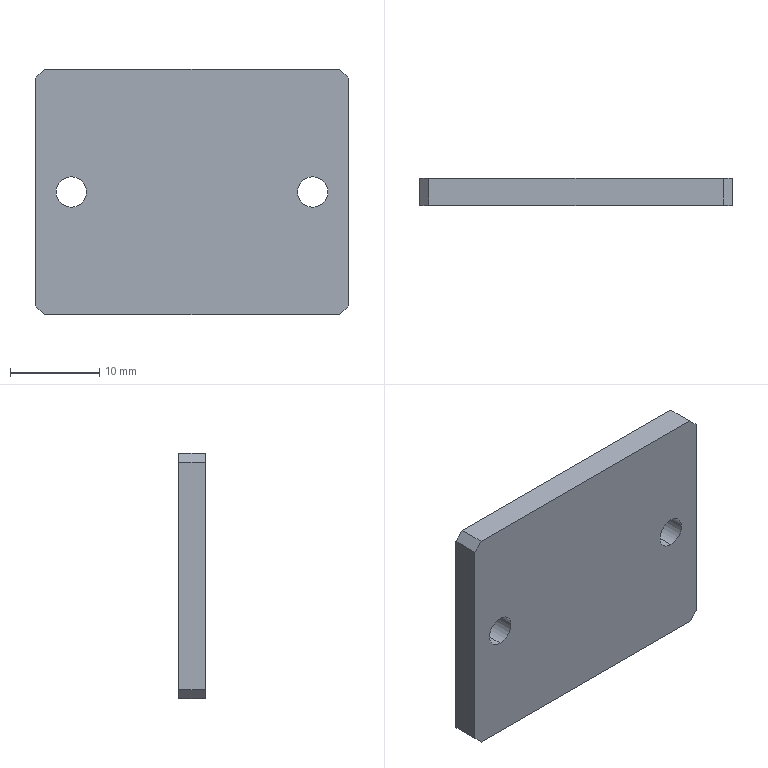Part | STEP file | PN_0050 | 1 solid | 14 faces | box 35 x 3 x 27.5 mm | volume 2827 mm3 | plane 10 | cylinder 4 | commonest cylinder face diameters 3.4 x4
STEP:
#1=CARTESIAN_POINT('',(0.,0.,0.));
#2=DIRECTION('',(0.,0.,1.));
#3=DIRECTION('',(1.,0.,0.));
#4=AXIS2_PLACEMENT_3D('',#1,#2,#3);
#5=CARTESIAN_POINT('',(13.5,0.,1.7));
#6=VERTEX_POINT('',#5);
#7=CARTESIAN_POINT('',(13.5,3.,1.7));
#8=VERTEX_POINT('',#7);
#9=CARTESIAN_POINT('',(13.5,0.,1.7));
#10=DIRECTION('',(0.,1.,0.));
#11=VECTOR('',#10,1.);
#12=LINE('',#9,#11);
#13=CARTESIAN_POINT('',(13.5,0.,0.));
#14=DIRECTION('',(0.,1.,0.));
#15=DIRECTION('',(0.,0.,1.));
#16=AXIS2_PLACEMENT_3D('',#13,#14,#15);
#17=CYLINDRICAL_SURFACE('',#16,1.7);
#18=CARTESIAN_POINT('',(6.283,0.));
#19=DIRECTION('',(0.,1.));
#20=VECTOR('',#19,1.);
#21=LINE('',#18,#20);
#22=(GEOMETRIC_REPRESENTATION_CONTEXT(2)PARAMETRIC_REPRESENTATION_CONTEXT()REPRESENTATION_CONTEXT('',''));
#23=DEFINITIONAL_REPRESENTATION('',(#21),#22);
#24=PCURVE('',#17,#23);
#25=CARTESIAN_POINT('',(13.5,0.,0.));
#26=DIRECTION('',(0.,1.,0.));
#27=DIRECTION('',(0.,0.,1.));
#28=AXIS2_PLACEMENT_3D('',#25,#26,#27);
#29=CYLINDRICAL_SURFACE('',#28,1.7);
#30=CARTESIAN_POINT('',(0.,0.));
#31=DIRECTION('',(0.,1.));
#32=VECTOR('',#31,1.);
#33=LINE('',#30,#32);
#34=(GEOMETRIC_REPRESENTATION_CONTEXT(2)PARAMETRIC_REPRESENTATION_CONTEXT()REPRESENTATION_CONTEXT('',''));
#35=DEFINITIONAL_REPRESENTATION('',(#33),#34);
#36=PCURVE('',#29,#35);
#37=SURFACE_CURVE('',#12,(#24,#36),.PCURVE_S1.);
#38=EDGE_CURVE('',#6,#8,#37,.T.);
#39=ORIENTED_EDGE('',*,*,#38,.T.);
#40=CARTESIAN_POINT('',(13.5,3.,-1.7));
#41=VERTEX_POINT('',#40);
#42=CARTESIAN_POINT('',(13.5,3.,0.));
#43=DIRECTION('',(0.,1.,0.));
#44=DIRECTION('',(0.,0.,1.));
#45=AXIS2_PLACEMENT_3D('',#42,#43,#44);
#46=CIRCLE('',#45,1.7);
#47=CARTESIAN_POINT('',(0.,3.));
#48=DIRECTION('',(1.,0.));
#49=VECTOR('',#48,1.);
#50=LINE('',#47,#49);
#51=(GEOMETRIC_REPRESENTATION_CONTEXT(2)PARAMETRIC_REPRESENTATION_CONTEXT()REPRESENTATION_CONTEXT('',''));
#52=DEFINITIONAL_REPRESENTATION('',(#50),#51);
#53=PCURVE('',#17,#52);
#54=CARTESIAN_POINT('',(0.,3.,0.));
#55=DIRECTION('',(0.,1.,0.));
#56=DIRECTION('',(0.,0.,1.));
#57=AXIS2_PLACEMENT_3D('',#54,#55,#56);
#58=PLANE('',#57);
#59=CARTESIAN_POINT('',(0.,13.5));
#60=DIRECTION('',(1.,0.));
#61=AXIS2_PLACEMENT_2D('',#59,#60);
#62=CIRCLE('',#61,1.7);
#63=(GEOMETRIC_REPRESENTATION_CONTEXT(2)PARAMETRIC_REPRESENTATION_CONTEXT()REPRESENTATION_CONTEXT('',''));
#64=DEFINITIONAL_REPRESENTATION('',(#62),#63);
#65=PCURVE('',#58,#64);
#66=SURFACE_CURVE('',#46,(#53,#65),.PCURVE_S1.);
#67=EDGE_CURVE('',#41,#8,#66,.T.);
#68=ORIENTED_EDGE('',*,*,#67,.F.);
#69=CARTESIAN_POINT('',(13.5,0.,-1.7));
#70=VERTEX_POINT('',#69);
#71=CARTESIAN_POINT('',(13.5,0.,-1.7));
#72=DIRECTION('',(0.,1.,0.));
#73=VECTOR('',#72,1.);
#74=LINE('',#71,#73);
#75=CARTESIAN_POINT('',(3.142,0.));
#76=DIRECTION('',(0.,1.));
#77=VECTOR('',#76,1.);
#78=LINE('',#75,#77);
#79=(GEOMETRIC_REPRESENTATION_CONTEXT(2)PARAMETRIC_REPRESENTATION_CONTEXT()REPRESENTATION_CONTEXT('',''));
#80=DEFINITIONAL_REPRESENTATION('',(#78),#79);
#81=PCURVE('',#17,#80);
#82=CARTESIAN_POINT('',(3.142,0.));
#83=DIRECTION('',(0.,1.));
#84=VECTOR('',#83,1.);
#85=LINE('',#82,#84);
#86=(GEOMETRIC_REPRESENTATION_CONTEXT(2)PARAMETRIC_REPRESENTATION_CONTEXT()REPRESENTATION_CONTEXT('',''));
#87=DEFINITIONAL_REPRESENTATION('',(#85),#86);
#88=PCURVE('',#29,#87);
#89=SURFACE_CURVE('',#74,(#81,#88),.PCURVE_S1.);
#90=EDGE_CURVE('',#70,#41,#89,.T.);
#91=ORIENTED_EDGE('',*,*,#90,.F.);
#92=CARTESIAN_POINT('',(13.5,0.,0.));
#93=DIRECTION('',(0.,1.,0.));
#94=DIRECTION('',(0.,0.,1.));
#95=AXIS2_PLACEMENT_3D('',#92,#93,#94);
#96=CIRCLE('',#95,1.7);
#97=CARTESIAN_POINT('',(0.,0.));
#98=DIRECTION('',(1.,0.));
#99=VECTOR('',#98,1.);
#100=LINE('',#97,#99);
#101=(GEOMETRIC_REPRESENTATION_CONTEXT(2)PARAMETRIC_REPRESENTATION_CONTEXT()REPRESENTATION_CONTEXT('',''));
#102=DEFINITIONAL_REPRESENTATION('',(#100),#101);
#103=PCURVE('',#17,#102);
#104=CARTESIAN_POINT('',(0.,0.,0.));
#105=DIRECTION('',(0.,1.,0.));
#106=DIRECTION('',(0.,0.,1.));
#107=AXIS2_PLACEMENT_3D('',#104,#105,#106);
#108=PLANE('',#107);
#109=CARTESIAN_POINT('',(0.,13.5));
#110=DIRECTION('',(1.,0.));
#111=AXIS2_PLACEMENT_2D('',#109,#110);
#112=CIRCLE('',#111,1.7);
#113=(GEOMETRIC_REPRESENTATION_CONTEXT(2)PARAMETRIC_REPRESENTATION_CONTEXT()REPRESENTATION_CONTEXT('',''));
#114=DEFINITIONAL_REPRESENTATION('',(#112),#113);
#115=PCURVE('',#108,#114);
#116=SURFACE_CURVE('',#96,(#103,#115),.PCURVE_S1.);
#117=EDGE_CURVE('',#70,#6,#116,.T.);
#118=ORIENTED_EDGE('',*,*,#117,.T.);
#119=EDGE_LOOP('',(#39,#68,#91,#118));
#120=FACE_BOUND('',#119,.F.);
#121=ADVANCED_FACE('',(#120),#17,.F.);
#122=CARTESIAN_POINT('',(-13.5,0.,1.7));
#123=VERTEX_POINT('',#122);
#124=CARTESIAN_POINT('',(-13.5,3.,1.7));
#125=VERTEX_POINT('',#124);
#126=CARTESIAN_POINT('',(-13.5,0.,1.7));
#127=DIRECTION('',(0.,1.,0.));
#128=VECTOR('',#127,1.);
#129=LINE('',#126,#128);
#130=CARTESIAN_POINT('',(-13.5,0.,0.));
#131=DIRECTION('',(0.,1.,0.));
#132=DIRECTION('',(0.,0.,1.));
#133=AXIS2_PLACEMENT_3D('',#130,#131,#132);
#134=CYLINDRICAL_SURFACE('',#133,1.7);
#135=CARTESIAN_POINT('',(6.283,0.));
#136=DIRECTION('',(0.,1.));
#137=VECTOR('',#136,1.);
#138=LINE('',#135,#137);
#139=(GEOMETRIC_REPRESENTATION_CONTEXT(2)PARAMETRIC_REPRESENTATION_CONTEXT()REPRESENTATION_CONTEXT('',''));
#140=DEFINITIONAL_REPRESENTATION('',(#138),#139);
#141=PCURVE('',#134,#140);
#142=CARTESIAN_POINT('',(-13.5,0.,0.));
#143=DIRECTION('',(0.,1.,0.));
#144=DIRECTION('',(0.,0.,1.));
#145=AXIS2_PLACEMENT_3D('',#142,#143,#144);
#146=CYLINDRICAL_SURFACE('',#145,1.7);
#147=CARTESIAN_POINT('',(0.,0.));
#148=DIRECTION('',(0.,1.));
#149=VECTOR('',#148,1.);
#150=LINE('',#147,#149);
#151=(GEOMETRIC_REPRESENTATION_CONTEXT(2)PARAMETRIC_REPRESENTATION_CONTEXT()REPRESENTATION_CONTEXT('',''));
#152=DEFINITIONAL_REPRESENTATION('',(#150),#151);
#153=PCURVE('',#146,#152);
#154=SURFACE_CURVE('',#129,(#141,#153),.PCURVE_S1.);
#155=EDGE_CURVE('',#123,#125,#154,.T.);
#156=ORIENTED_EDGE('',*,*,#155,.T.);
#157=CARTESIAN_POINT('',(-13.5,3.,-1.7));
#158=VERTEX_POINT('',#157);
#159=CARTESIAN_POINT('',(-13.5,3.,0.));
#160=DIRECTION('',(0.,1.,0.));
#161=DIRECTION('',(0.,0.,1.));
#162=AXIS2_PLACEMENT_3D('',#159,#160,#161);
#163=CIRCLE('',#162,1.7);
#164=CARTESIAN_POINT('',(0.,3.));
#165=DIRECTION('',(1.,0.));
#166=VECTOR('',#165,1.);
#167=LINE('',#164,#166);
#168=(GEOMETRIC_REPRESENTATION_CONTEXT(2)PARAMETRIC_REPRESENTATION_CONTEXT()REPRESENTATION_CONTEXT('',''));
#169=DEFINITIONAL_REPRESENTATION('',(#167),#168);
#170=PCURVE('',#134,#169);
#171=CARTESIAN_POINT('',(0.,-13.5));
#172=DIRECTION('',(1.,0.));
#173=AXIS2_PLACEMENT_2D('',#171,#172);
#174=CIRCLE('',#173,1.7);
#175=(GEOMETRIC_REPRESENTATION_CONTEXT(2)PARAMETRIC_REPRESENTATION_CONTEXT()REPRESENTATION_CONTEXT('',''));
#176=DEFINITIONAL_REPRESENTATION('',(#174),#175);
#177=PCURVE('',#58,#176);
#178=SURFACE_CURVE('',#163,(#170,#177),.PCURVE_S1.);
#179=EDGE_CURVE('',#158,#125,#178,.T.);
#180=ORIENTED_EDGE('',*,*,#179,.F.);
#181=CARTESIAN_POINT('',(-13.5,0.,-1.7));
#182=VERTEX_POINT('',#181);
#183=CARTESIAN_POINT('',(-13.5,0.,-1.7));
#184=DIRECTION('',(0.,1.,0.));
#185=VECTOR('',#184,1.);
#186=LINE('',#183,#185);
#187=CARTESIAN_POINT('',(3.142,0.));
#188=DIRECTION('',(0.,1.));
#189=VECTOR('',#188,1.);
#190=LINE('',#187,#189);
#191=(GEOMETRIC_REPRESENTATION_CONTEXT(2)PARAMETRIC_REPRESENTATION_CONTEXT()REPRESENTATION_CONTEXT('',''));
#192=DEFINITIONAL_REPRESENTATION('',(#190),#191);
#193=PCURVE('',#134,#192);
#194=CARTESIAN_POINT('',(3.142,0.));
#195=DIRECTION('',(0.,1.));
#196=VECTOR('',#195,1.);
#197=LINE('',#194,#196);
#198=(GEOMETRIC_REPRESENTATION_CONTEXT(2)PARAMETRIC_REPRESENTATION_CONTEXT()REPRESENTATION_CONTEXT('',''));
#199=DEFINITIONAL_REPRESENTATION('',(#197),#198);
#200=PCURVE('',#146,#199);
#201=SURFACE_CURVE('',#186,(#193,#200),.PCURVE_S1.);
#202=EDGE_CURVE('',#182,#158,#201,.T.);
#203=ORIENTED_EDGE('',*,*,#202,.F.);
#204=CARTESIAN_POINT('',(-13.5,0.,0.));
#205=DIRECTION('',(0.,1.,0.));
#206=DIRECTION('',(0.,0.,1.));
#207=AXIS2_PLACEMENT_3D('',#204,#205,#206);
#208=CIRCLE('',#207,1.7);
#209=CARTESIAN_POINT('',(0.,0.));
#210=DIRECTION('',(1.,0.));
#211=VECTOR('',#210,1.);
#212=LINE('',#209,#211);
#213=(GEOMETRIC_REPRESENTATION_CONTEXT(2)PARAMETRIC_REPRESENTATION_CONTEXT()REPRESENTATION_CONTEXT('',''));
#214=DEFINITIONAL_REPRESENTATION('',(#212),#213);
#215=PCURVE('',#134,#214);
#216=CARTESIAN_POINT('',(0.,-13.5));
#217=DIRECTION('',(1.,0.));
#218=AXIS2_PLACEMENT_2D('',#216,#217);
#219=CIRCLE('',#218,1.7);
#220=(GEOMETRIC_REPRESENTATION_CONTEXT(2)PARAMETRIC_REPRESENTATION_CONTEXT()REPRESENTATION_CONTEXT('',''));
#221=DEFINITIONAL_REPRESENTATION('',(#219),#220);
#222=PCURVE('',#108,#221);
#223=SURFACE_CURVE('',#208,(#215,#222),.PCURVE_S1.);
#224=EDGE_CURVE('',#182,#123,#223,.T.);
#225=ORIENTED_EDGE('',*,*,#224,.T.);
#226=EDGE_LOOP('',(#156,#180,#203,#225));
#227=FACE_BOUND('',#226,.F.);
#228=ADVANCED_FACE('',(#227),#134,.F.);
#229=CARTESIAN_POINT('',(17.5,0.,12.75));
#230=VERTEX_POINT('',#229);
#231=CARTESIAN_POINT('',(17.5,0.,-12.75));
#232=VERTEX_POINT('',#231);
#233=CARTESIAN_POINT('',(17.5,0.,-13.75));
#234=DIRECTION('',(0.,0.,-1.));
#235=VECTOR('',#234,1.);
#236=LINE('',#233,#235);
#237=CARTESIAN_POINT('',(17.5,3.,-13.75));
#238=DIRECTION('',(-1.,0.,0.));
#239=DIRECTION('',(0.,0.,1.));
#240=AXIS2_PLACEMENT_3D('',#237,#238,#239);
#241=PLANE('',#240);
#242=CARTESIAN_POINT('',(0.,-3.));
#243=DIRECTION('',(-1.,0.));
#244=VECTOR('',#243,1.);
#245=LINE('',#242,#244);
#246=(GEOMETRIC_REPRESENTATION_CONTEXT(2)PARAMETRIC_REPRESENTATION_CONTEXT()REPRESENTATION_CONTEXT('',''));
#247=DEFINITIONAL_REPRESENTATION('',(#245),#246);
#248=PCURVE('',#241,#247);
#249=CARTESIAN_POINT('',(-13.75,17.5));
#250=DIRECTION('',(-1.,0.));
#251=VECTOR('',#250,1.);
#252=LINE('',#249,#251);
#253=(GEOMETRIC_REPRESENTATION_CONTEXT(2)PARAMETRIC_REPRESENTATION_CONTEXT()REPRESENTATION_CONTEXT('',''));
#254=DEFINITIONAL_REPRESENTATION('',(#252),#253);
#255=PCURVE('',#108,#254);
#256=SURFACE_CURVE('',#236,(#248,#255),.PCURVE_S1.);
#257=EDGE_CURVE('',#230,#232,#256,.T.);
#258=ORIENTED_EDGE('',*,*,#257,.T.);
#259=CARTESIAN_POINT('',(17.5,3.,-12.75));
#260=VERTEX_POINT('',#259);
#261=CARTESIAN_POINT('',(17.5,3.,-12.75));
#262=DIRECTION('',(0.,1.,0.));
#263=VECTOR('',#262,1.);
#264=LINE('',#261,#263);
#265=CARTESIAN_POINT('',(1.,0.));
#266=DIRECTION('',(0.,1.));
#267=VECTOR('',#266,1.);
#268=LINE('',#265,#267);
#269=(GEOMETRIC_REPRESENTATION_CONTEXT(2)PARAMETRIC_REPRESENTATION_CONTEXT()REPRESENTATION_CONTEXT('',''));
#270=DEFINITIONAL_REPRESENTATION('',(#268),#269);
#271=PCURVE('',#241,#270);
#272=CARTESIAN_POINT('',(16.5,3.,-13.75));
#273=DIRECTION('',(-0.7071,0.,0.7071));
#274=DIRECTION('',(0.,-1.,0.));
#275=AXIS2_PLACEMENT_3D('',#272,#273,#274);
#276=PLANE('',#275);
#277=CARTESIAN_POINT('',(0.,1.414));
#278=DIRECTION('',(-1.,0.));
#279=VECTOR('',#278,1.);
#280=LINE('',#277,#279);
#281=(GEOMETRIC_REPRESENTATION_CONTEXT(2)PARAMETRIC_REPRESENTATION_CONTEXT()REPRESENTATION_CONTEXT('',''));
#282=DEFINITIONAL_REPRESENTATION('',(#280),#281);
#283=PCURVE('',#276,#282);
#284=SURFACE_CURVE('',#264,(#271,#283),.PCURVE_S1.);
#285=EDGE_CURVE('',#232,#260,#284,.T.);
#286=ORIENTED_EDGE('',*,*,#285,.T.);
#287=CARTESIAN_POINT('',(17.5,3.,12.75));
#288=VERTEX_POINT('',#287);
#289=CARTESIAN_POINT('',(17.5,3.,-13.75));
#290=DIRECTION('',(0.,0.,-1.));
#291=VECTOR('',#290,1.);
#292=LINE('',#289,#291);
#293=CARTESIAN_POINT('',(0.,0.));
#294=DIRECTION('',(-1.,0.));
#295=VECTOR('',#294,1.);
#296=LINE('',#293,#295);
#297=(GEOMETRIC_REPRESENTATION_CONTEXT(2)PARAMETRIC_REPRESENTATION_CONTEXT()REPRESENTATION_CONTEXT('',''));
#298=DEFINITIONAL_REPRESENTATION('',(#296),#297);
#299=PCURVE('',#241,#298);
#300=CARTESIAN_POINT('',(-13.75,17.5));
#301=DIRECTION('',(-1.,0.));
#302=VECTOR('',#301,1.);
#303=LINE('',#300,#302);
#304=(GEOMETRIC_REPRESENTATION_CONTEXT(2)PARAMETRIC_REPRESENTATION_CONTEXT()REPRESENTATION_CONTEXT('',''));
#305=DEFINITIONAL_REPRESENTATION('',(#303),#304);
#306=PCURVE('',#58,#305);
#307=SURFACE_CURVE('',#292,(#299,#306),.PCURVE_S1.);
#308=EDGE_CURVE('',#288,#260,#307,.T.);
#309=ORIENTED_EDGE('',*,*,#308,.F.);
#310=CARTESIAN_POINT('',(17.5,3.,12.75));
#311=DIRECTION('',(0.,-1.,0.));
#312=VECTOR('',#311,1.);
#313=LINE('',#310,#312);
#314=CARTESIAN_POINT('',(26.5,0.));
#315=DIRECTION('',(0.,-1.));
#316=VECTOR('',#315,1.);
#317=LINE('',#314,#316);
#318=(GEOMETRIC_REPRESENTATION_CONTEXT(2)PARAMETRIC_REPRESENTATION_CONTEXT()REPRESENTATION_CONTEXT('',''));
#319=DEFINITIONAL_REPRESENTATION('',(#317),#318);
#320=PCURVE('',#241,#319);
#321=CARTESIAN_POINT('',(17.5,3.,12.75));
#322=DIRECTION('',(-0.7071,0.,-0.7071));
#323=DIRECTION('',(0.,-1.,0.));
#324=AXIS2_PLACEMENT_3D('',#321,#322,#323);
#325=PLANE('',#324);
#326=CARTESIAN_POINT('',(0.,0.));
#327=DIRECTION('',(1.,0.));
#328=VECTOR('',#327,1.);
#329=LINE('',#326,#328);
#330=(GEOMETRIC_REPRESENTATION_CONTEXT(2)PARAMETRIC_REPRESENTATION_CONTEXT()REPRESENTATION_CONTEXT('',''));
#331=DEFINITIONAL_REPRESENTATION('',(#329),#330);
#332=PCURVE('',#325,#331);
#333=SURFACE_CURVE('',#313,(#320,#332),.PCURVE_S1.);
#334=EDGE_CURVE('',#288,#230,#333,.T.);
#335=ORIENTED_EDGE('',*,*,#334,.T.);
#336=EDGE_LOOP('',(#258,#286,#309,#335));
#337=FACE_BOUND('',#336,.T.);
#338=ADVANCED_FACE('',(#337),#241,.F.);
#339=CARTESIAN_POINT('',(16.5,3.,-13.75));
#340=VERTEX_POINT('',#339);
#341=CARTESIAN_POINT('',(-16.5,3.,-13.75));
#342=VERTEX_POINT('',#341);
#343=CARTESIAN_POINT('',(-17.5,3.,-13.75));
#344=DIRECTION('',(-1.,0.,0.));
#345=VECTOR('',#344,1.);
#346=LINE('',#343,#345);
#347=CARTESIAN_POINT('',(-17.5,3.,-13.75));
#348=DIRECTION('',(0.,0.,1.));
#349=DIRECTION('',(1.,0.,0.));
#350=AXIS2_PLACEMENT_3D('',#347,#348,#349);
#351=PLANE('',#350);
#352=CARTESIAN_POINT('',(0.,0.));
#353=DIRECTION('',(-1.,0.));
#354=VECTOR('',#353,1.);
#355=LINE('',#352,#354);
#356=(GEOMETRIC_REPRESENTATION_CONTEXT(2)PARAMETRIC_REPRESENTATION_CONTEXT()REPRESENTATION_CONTEXT('',''));
#357=DEFINITIONAL_REPRESENTATION('',(#355),#356);
#358=PCURVE('',#351,#357);
#359=CARTESIAN_POINT('',(-13.75,-17.5));
#360=DIRECTION('',(0.,-1.));
#361=VECTOR('',#360,1.);
#362=LINE('',#359,#361);
#363=(GEOMETRIC_REPRESENTATION_CONTEXT(2)PARAMETRIC_REPRESENTATION_CONTEXT()REPRESENTATION_CONTEXT('',''));
#364=DEFINITIONAL_REPRESENTATION('',(#362),#363);
#365=PCURVE('',#58,#364);
#366=SURFACE_CURVE('',#346,(#358,#365),.PCURVE_S1.);
#367=EDGE_CURVE('',#340,#342,#366,.T.);
#368=ORIENTED_EDGE('',*,*,#367,.F.);
#369=CARTESIAN_POINT('',(16.5,0.,-13.75));
#370=VERTEX_POINT('',#369);
#371=CARTESIAN_POINT('',(16.5,3.,-13.75));
#372=DIRECTION('',(0.,-1.,0.));
#373=VECTOR('',#372,1.);
#374=LINE('',#371,#373);
#375=CARTESIAN_POINT('',(34.,0.));
#376=DIRECTION('',(0.,-1.));
#377=VECTOR('',#376,1.);
#378=LINE('',#375,#377);
#379=(GEOMETRIC_REPRESENTATION_CONTEXT(2)PARAMETRIC_REPRESENTATION_CONTEXT()REPRESENTATION_CONTEXT('',''));
#380=DEFINITIONAL_REPRESENTATION('',(#378),#379);
#381=PCURVE('',#351,#380);
#382=CARTESIAN_POINT('',(0.,0.));
#383=DIRECTION('',(1.,0.));
#384=VECTOR('',#383,1.);
#385=LINE('',#382,#384);
#386=(GEOMETRIC_REPRESENTATION_CONTEXT(2)PARAMETRIC_REPRESENTATION_CONTEXT()REPRESENTATION_CONTEXT('',''));
#387=DEFINITIONAL_REPRESENTATION('',(#385),#386);
#388=PCURVE('',#276,#387);
#389=SURFACE_CURVE('',#374,(#381,#388),.PCURVE_S1.);
#390=EDGE_CURVE('',#340,#370,#389,.T.);
#391=ORIENTED_EDGE('',*,*,#390,.T.);
#392=CARTESIAN_POINT('',(-16.5,0.,-13.75));
#393=VERTEX_POINT('',#392);
#394=CARTESIAN_POINT('',(-17.5,0.,-13.75));
#395=DIRECTION('',(-1.,0.,0.));
#396=VECTOR('',#395,1.);
#397=LINE('',#394,#396);
#398=CARTESIAN_POINT('',(0.,-3.));
#399=DIRECTION('',(-1.,0.));
#400=VECTOR('',#399,1.);
#401=LINE('',#398,#400);
#402=(GEOMETRIC_REPRESENTATION_CONTEXT(2)PARAMETRIC_REPRESENTATION_CONTEXT()REPRESENTATION_CONTEXT('',''));
#403=DEFINITIONAL_REPRESENTATION('',(#401),#402);
#404=PCURVE('',#351,#403);
#405=CARTESIAN_POINT('',(-13.75,-17.5));
#406=DIRECTION('',(0.,-1.));
#407=VECTOR('',#406,1.);
#408=LINE('',#405,#407);
#409=(GEOMETRIC_REPRESENTATION_CONTEXT(2)PARAMETRIC_REPRESENTATION_CONTEXT()REPRESENTATION_CONTEXT('',''));
#410=DEFINITIONAL_REPRESENTATION('',(#408),#409);
#411=PCURVE('',#108,#410);
#412=SURFACE_CURVE('',#397,(#404,#411),.PCURVE_S1.);
#413=EDGE_CURVE('',#370,#393,#412,.T.);
#414=ORIENTED_EDGE('',*,*,#413,.T.);
#415=CARTESIAN_POINT('',(-16.5,3.,-13.75));
#416=DIRECTION('',(0.,1.,0.));
#417=VECTOR('',#416,1.);
#418=LINE('',#415,#417);
#419=CARTESIAN_POINT('',(1.,0.));
#420=DIRECTION('',(0.,1.));
#421=VECTOR('',#420,1.);
#422=LINE('',#419,#421);
#423=(GEOMETRIC_REPRESENTATION_CONTEXT(2)PARAMETRIC_REPRESENTATION_CONTEXT()REPRESENTATION_CONTEXT('',''));
#424=DEFINITIONAL_REPRESENTATION('',(#422),#423);
#425=PCURVE('',#351,#424);
#426=CARTESIAN_POINT('',(-17.5,3.,-12.75));
#427=DIRECTION('',(0.7071,0.,0.7071));
#428=DIRECTION('',(0.,-1.,0.));
#429=AXIS2_PLACEMENT_3D('',#426,#427,#428);
#430=PLANE('',#429);
#431=CARTESIAN_POINT('',(0.,1.414));
#432=DIRECTION('',(-1.,0.));
#433=VECTOR('',#432,1.);
#434=LINE('',#431,#433);
#435=(GEOMETRIC_REPRESENTATION_CONTEXT(2)PARAMETRIC_REPRESENTATION_CONTEXT()REPRESENTATION_CONTEXT('',''));
#436=DEFINITIONAL_REPRESENTATION('',(#434),#435);
#437=PCURVE('',#430,#436);
#438=SURFACE_CURVE('',#418,(#425,#437),.PCURVE_S1.);
#439=EDGE_CURVE('',#393,#342,#438,.T.);
#440=ORIENTED_EDGE('',*,*,#439,.T.);
#441=EDGE_LOOP('',(#368,#391,#414,#440));
#442=FACE_BOUND('',#441,.T.);
#443=ADVANCED_FACE('',(#442),#351,.F.);
#444=CARTESIAN_POINT('',(-17.5,3.,-12.75));
#445=VERTEX_POINT('',#444);
#446=CARTESIAN_POINT('',(-17.5,3.,12.75));
#447=VERTEX_POINT('',#446);
#448=CARTESIAN_POINT('',(-17.5,3.,-13.75));
#449=DIRECTION('',(0.,0.,1.));
#450=VECTOR('',#449,1.);
#451=LINE('',#448,#450);
#452=CARTESIAN_POINT('',(-17.5,3.,-13.75));
#453=DIRECTION('',(1.,0.,0.));
#454=DIRECTION('',(0.,0.,-1.));
#455=AXIS2_PLACEMENT_3D('',#452,#453,#454);
#456=PLANE('',#455);
#457=CARTESIAN_POINT('',(0.,0.));
#458=DIRECTION('',(-1.,0.));
#459=VECTOR('',#458,1.);
#460=LINE('',#457,#459);
#461=(GEOMETRIC_REPRESENTATION_CONTEXT(2)PARAMETRIC_REPRESENTATION_CONTEXT()REPRESENTATION_CONTEXT('',''));
#462=DEFINITIONAL_REPRESENTATION('',(#460),#461);
#463=PCURVE('',#456,#462);
#464=CARTESIAN_POINT('',(-13.75,-17.5));
#465=DIRECTION('',(1.,0.));
#466=VECTOR('',#465,1.);
#467=LINE('',#464,#466);
#468=(GEOMETRIC_REPRESENTATION_CONTEXT(2)PARAMETRIC_REPRESENTATION_CONTEXT()REPRESENTATION_CONTEXT('',''));
#469=DEFINITIONAL_REPRESENTATION('',(#467),#468);
#470=PCURVE('',#58,#469);
#471=SURFACE_CURVE('',#451,(#463,#470),.PCURVE_S1.);
#472=EDGE_CURVE('',#445,#447,#471,.T.);
#473=ORIENTED_EDGE('',*,*,#472,.F.);
#474=CARTESIAN_POINT('',(-17.5,0.,-12.75));
#475=VERTEX_POINT('',#474);
#476=CARTESIAN_POINT('',(-17.5,3.,-12.75));
#477=DIRECTION('',(0.,-1.,0.));
#478=VECTOR('',#477,1.);
#479=LINE('',#476,#478);
#480=CARTESIAN_POINT('',(-1.,0.));
#481=DIRECTION('',(0.,-1.));
#482=VECTOR('',#481,1.);
#483=LINE('',#480,#482);
#484=(GEOMETRIC_REPRESENTATION_CONTEXT(2)PARAMETRIC_REPRESENTATION_CONTEXT()REPRESENTATION_CONTEXT('',''));
#485=DEFINITIONAL_REPRESENTATION('',(#483),#484);
#486=PCURVE('',#456,#485);
#487=CARTESIAN_POINT('',(0.,0.));
#488=DIRECTION('',(1.,0.));
#489=VECTOR('',#488,1.);
#490=LINE('',#487,#489);
#491=(GEOMETRIC_REPRESENTATION_CONTEXT(2)PARAMETRIC_REPRESENTATION_CONTEXT()REPRESENTATION_CONTEXT('',''));
#492=DEFINITIONAL_REPRESENTATION('',(#490),#491);
#493=PCURVE('',#430,#492);
#494=SURFACE_CURVE('',#479,(#486,#493),.PCURVE_S1.);
#495=EDGE_CURVE('',#445,#475,#494,.T.);
#496=ORIENTED_EDGE('',*,*,#495,.T.);
#497=CARTESIAN_POINT('',(-17.5,0.,12.75));
#498=VERTEX_POINT('',#497);
#499=CARTESIAN_POINT('',(-17.5,0.,-13.75));
#500=DIRECTION('',(0.,0.,1.));
#501=VECTOR('',#500,1.);
#502=LINE('',#499,#501);
#503=CARTESIAN_POINT('',(0.,-3.));
#504=DIRECTION('',(-1.,0.));
#505=VECTOR('',#504,1.);
#506=LINE('',#503,#505);
#507=(GEOMETRIC_REPRESENTATION_CONTEXT(2)PARAMETRIC_REPRESENTATION_CONTEXT()REPRESENTATION_CONTEXT('',''));
#508=DEFINITIONAL_REPRESENTATION('',(#506),#507);
#509=PCURVE('',#456,#508);
#510=CARTESIAN_POINT('',(-13.75,-17.5));
#511=DIRECTION('',(1.,0.));
#512=VECTOR('',#511,1.);
#513=LINE('',#510,#512);
#514=(GEOMETRIC_REPRESENTATION_CONTEXT(2)PARAMETRIC_REPRESENTATION_CONTEXT()REPRESENTATION_CONTEXT('',''));
#515=DEFINITIONAL_REPRESENTATION('',(#513),#514);
#516=PCURVE('',#108,#515);
#517=SURFACE_CURVE('',#502,(#509,#516),.PCURVE_S1.);
#518=EDGE_CURVE('',#475,#498,#517,.T.);
#519=ORIENTED_EDGE('',*,*,#518,.T.);
#520=CARTESIAN_POINT('',(-17.5,3.,12.75));
#521=DIRECTION('',(0.,1.,0.));
#522=VECTOR('',#521,1.);
#523=LINE('',#520,#522);
#524=CARTESIAN_POINT('',(-26.5,0.));
#525=DIRECTION('',(0.,1.));
#526=VECTOR('',#525,1.);
#527=LINE('',#524,#526);
#528=(GEOMETRIC_REPRESENTATION_CONTEXT(2)PARAMETRIC_REPRESENTATION_CONTEXT()REPRESENTATION_CONTEXT('',''));
#529=DEFINITIONAL_REPRESENTATION('',(#527),#528);
#530=PCURVE('',#456,#529);
#531=CARTESIAN_POINT('',(-16.5,3.,13.75));
#532=DIRECTION('',(0.7071,0.,-0.7071));
#533=DIRECTION('',(0.,-1.,0.));
#534=AXIS2_PLACEMENT_3D('',#531,#532,#533);
#535=PLANE('',#534);
#536=CARTESIAN_POINT('',(0.,1.414));
#537=DIRECTION('',(-1.,0.));
#538=VECTOR('',#537,1.);
#539=LINE('',#536,#538);
#540=(GEOMETRIC_REPRESENTATION_CONTEXT(2)PARAMETRIC_REPRESENTATION_CONTEXT()REPRESENTATION_CONTEXT('',''));
#541=DEFINITIONAL_REPRESENTATION('',(#539),#540);
#542=PCURVE('',#535,#541);
#543=SURFACE_CURVE('',#523,(#530,#542),.PCURVE_S1.);
#544=EDGE_CURVE('',#498,#447,#543,.T.);
#545=ORIENTED_EDGE('',*,*,#544,.T.);
#546=EDGE_LOOP('',(#473,#496,#519,#545));
#547=FACE_BOUND('',#546,.T.);
#548=ADVANCED_FACE('',(#547),#456,.F.);
#549=CARTESIAN_POINT('',(-16.5,0.,13.75));
#550=VERTEX_POINT('',#549);
#551=CARTESIAN_POINT('',(16.5,0.,13.75));
#552=VERTEX_POINT('',#551);
#553=CARTESIAN_POINT('',(-17.5,0.,13.75));
#554=DIRECTION('',(1.,0.,0.));
#555=VECTOR('',#554,1.);
#556=LINE('',#553,#555);
#557=CARTESIAN_POINT('',(-17.5,3.,13.75));
#558=DIRECTION('',(0.,0.,-1.));
#559=DIRECTION('',(-1.,0.,0.));
#560=AXIS2_PLACEMENT_3D('',#557,#558,#559);
#561=PLANE('',#560);
#562=CARTESIAN_POINT('',(0.,-3.));
#563=DIRECTION('',(-1.,0.));
#564=VECTOR('',#563,1.);
#565=LINE('',#562,#564);
#566=(GEOMETRIC_REPRESENTATION_CONTEXT(2)PARAMETRIC_REPRESENTATION_CONTEXT()REPRESENTATION_CONTEXT('',''));
#567=DEFINITIONAL_REPRESENTATION('',(#565),#566);
#568=PCURVE('',#561,#567);
#569=CARTESIAN_POINT('',(13.75,-17.5));
#570=DIRECTION('',(0.,1.));
#571=VECTOR('',#570,1.);
#572=LINE('',#569,#571);
#573=(GEOMETRIC_REPRESENTATION_CONTEXT(2)PARAMETRIC_REPRESENTATION_CONTEXT()REPRESENTATION_CONTEXT('',''));
#574=DEFINITIONAL_REPRESENTATION('',(#572),#573);
#575=PCURVE('',#108,#574);
#576=SURFACE_CURVE('',#556,(#568,#575),.PCURVE_S1.);
#577=EDGE_CURVE('',#550,#552,#576,.T.);
#578=ORIENTED_EDGE('',*,*,#577,.T.);
#579=CARTESIAN_POINT('',(16.5,3.,13.75));
#580=VERTEX_POINT('',#579);
#581=CARTESIAN_POINT('',(16.5,3.,13.75));
#582=DIRECTION('',(0.,1.,0.));
#583=VECTOR('',#582,1.);
#584=LINE('',#581,#583);
#585=CARTESIAN_POINT('',(-34.,0.));
#586=DIRECTION('',(0.,1.));
#587=VECTOR('',#586,1.);
#588=LINE('',#585,#587);
#589=(GEOMETRIC_REPRESENTATION_CONTEXT(2)PARAMETRIC_REPRESENTATION_CONTEXT()REPRESENTATION_CONTEXT('',''));
#590=DEFINITIONAL_REPRESENTATION('',(#588),#589);
#591=PCURVE('',#561,#590);
#592=CARTESIAN_POINT('',(0.,1.414));
#593=DIRECTION('',(-1.,0.));
#594=VECTOR('',#593,1.);
#595=LINE('',#592,#594);
#596=(GEOMETRIC_REPRESENTATION_CONTEXT(2)PARAMETRIC_REPRESENTATION_CONTEXT()REPRESENTATION_CONTEXT('',''));
#597=DEFINITIONAL_REPRESENTATION('',(#595),#596);
#598=PCURVE('',#325,#597);
#599=SURFACE_CURVE('',#584,(#591,#598),.PCURVE_S1.);
#600=EDGE_CURVE('',#552,#580,#599,.T.);
#601=ORIENTED_EDGE('',*,*,#600,.T.);
#602=CARTESIAN_POINT('',(-16.5,3.,13.75));
#603=VERTEX_POINT('',#602);
#604=CARTESIAN_POINT('',(-17.5,3.,13.75));
#605=DIRECTION('',(1.,0.,0.));
#606=VECTOR('',#605,1.);
#607=LINE('',#604,#606);
#608=CARTESIAN_POINT('',(0.,0.));
#609=DIRECTION('',(-1.,0.));
#610=VECTOR('',#609,1.);
#611=LINE('',#608,#610);
#612=(GEOMETRIC_REPRESENTATION_CONTEXT(2)PARAMETRIC_REPRESENTATION_CONTEXT()REPRESENTATION_CONTEXT('',''));
#613=DEFINITIONAL_REPRESENTATION('',(#611),#612);
#614=PCURVE('',#561,#613);
#615=CARTESIAN_POINT('',(13.75,-17.5));
#616=DIRECTION('',(0.,1.));
#617=VECTOR('',#616,1.);
#618=LINE('',#615,#617);
#619=(GEOMETRIC_REPRESENTATION_CONTEXT(2)PARAMETRIC_REPRESENTATION_CONTEXT()REPRESENTATION_CONTEXT('',''));
#620=DEFINITIONAL_REPRESENTATION('',(#618),#619);
#621=PCURVE('',#58,#620);
#622=SURFACE_CURVE('',#607,(#614,#621),.PCURVE_S1.);
#623=EDGE_CURVE('',#603,#580,#622,.T.);
#624=ORIENTED_EDGE('',*,*,#623,.F.);
#625=CARTESIAN_POINT('',(-16.5,3.,13.75));
#626=DIRECTION('',(0.,-1.,0.));
#627=VECTOR('',#626,1.);
#628=LINE('',#625,#627);
#629=CARTESIAN_POINT('',(-1.,0.));
#630=DIRECTION('',(0.,-1.));
#631=VECTOR('',#630,1.);
#632=LINE('',#629,#631);
#633=(GEOMETRIC_REPRESENTATION_CONTEXT(2)PARAMETRIC_REPRESENTATION_CONTEXT()REPRESENTATION_CONTEXT('',''));
#634=DEFINITIONAL_REPRESENTATION('',(#632),#633);
#635=PCURVE('',#561,#634);
#636=CARTESIAN_POINT('',(0.,0.));
#637=DIRECTION('',(1.,0.));
#638=VECTOR('',#637,1.);
#639=LINE('',#636,#638);
#640=(GEOMETRIC_REPRESENTATION_CONTEXT(2)PARAMETRIC_REPRESENTATION_CONTEXT()REPRESENTATION_CONTEXT('',''));
#641=DEFINITIONAL_REPRESENTATION('',(#639),#640);
#642=PCURVE('',#535,#641);
#643=SURFACE_CURVE('',#628,(#635,#642),.PCURVE_S1.);
#644=EDGE_CURVE('',#603,#550,#643,.T.);
#645=ORIENTED_EDGE('',*,*,#644,.T.);
#646=EDGE_LOOP('',(#578,#601,#624,#645));
#647=FACE_BOUND('',#646,.T.);
#648=ADVANCED_FACE('',(#647),#561,.F.);
#649=CARTESIAN_POINT('',(13.5,3.,0.));
#650=DIRECTION('',(0.,1.,0.));
#651=DIRECTION('',(0.,0.,1.));
#652=AXIS2_PLACEMENT_3D('',#649,#650,#651);
#653=CIRCLE('',#652,1.7);
#654=CARTESIAN_POINT('',(0.,13.5));
#655=DIRECTION('',(1.,0.));
#656=AXIS2_PLACEMENT_2D('',#654,#655);
#657=CIRCLE('',#656,1.7);
#658=(GEOMETRIC_REPRESENTATION_CONTEXT(2)PARAMETRIC_REPRESENTATION_CONTEXT()REPRESENTATION_CONTEXT('',''));
#659=DEFINITIONAL_REPRESENTATION('',(#657),#658);
#660=PCURVE('',#58,#659);
#661=CARTESIAN_POINT('',(0.,3.));
#662=DIRECTION('',(1.,0.));
#663=VECTOR('',#662,1.);
#664=LINE('',#661,#663);
#665=(GEOMETRIC_REPRESENTATION_CONTEXT(2)PARAMETRIC_REPRESENTATION_CONTEXT()REPRESENTATION_CONTEXT('',''));
#666=DEFINITIONAL_REPRESENTATION('',(#664),#665);
#667=PCURVE('',#29,#666);
#668=SURFACE_CURVE('',#653,(#660,#667),.PCURVE_S1.);
#669=EDGE_CURVE('',#8,#41,#668,.T.);
#670=ORIENTED_EDGE('',*,*,#669,.F.);
#671=ORIENTED_EDGE('',*,*,#67,.F.);
#672=EDGE_LOOP('',(#670,#671));
#673=FACE_BOUND('',#672,.T.);
#674=CARTESIAN_POINT('',(-13.5,3.,0.));
#675=DIRECTION('',(0.,1.,0.));
#676=DIRECTION('',(0.,0.,1.));
#677=AXIS2_PLACEMENT_3D('',#674,#675,#676);
#678=CIRCLE('',#677,1.7);
#679=CARTESIAN_POINT('',(0.,-13.5));
#680=DIRECTION('',(1.,0.));
#681=AXIS2_PLACEMENT_2D('',#679,#680);
#682=CIRCLE('',#681,1.7);
#683=(GEOMETRIC_REPRESENTATION_CONTEXT(2)PARAMETRIC_REPRESENTATION_CONTEXT()REPRESENTATION_CONTEXT('',''));
#684=DEFINITIONAL_REPRESENTATION('',(#682),#683);
#685=PCURVE('',#58,#684);
#686=CARTESIAN_POINT('',(0.,3.));
#687=DIRECTION('',(1.,0.));
#688=VECTOR('',#687,1.);
#689=LINE('',#686,#688);
#690=(GEOMETRIC_REPRESENTATION_CONTEXT(2)PARAMETRIC_REPRESENTATION_CONTEXT()REPRESENTATION_CONTEXT('',''));
#691=DEFINITIONAL_REPRESENTATION('',(#689),#690);
#692=PCURVE('',#146,#691);
#693=SURFACE_CURVE('',#678,(#685,#692),.PCURVE_S1.);
#694=EDGE_CURVE('',#125,#158,#693,.T.);
#695=ORIENTED_EDGE('',*,*,#694,.F.);
#696=ORIENTED_EDGE('',*,*,#179,.F.);
#697=EDGE_LOOP('',(#695,#696));
#698=FACE_BOUND('',#697,.T.);
#699=ORIENTED_EDGE('',*,*,#308,.T.);
#700=CARTESIAN_POINT('',(15.125,3.,-15.125));
#701=DIRECTION('',(-0.7071,0.,-0.7071));
#702=VECTOR('',#701,1.);
#703=LINE('',#700,#702);
#704=CARTESIAN_POINT('',(-15.125,15.125));
#705=DIRECTION('',(-0.7071,-0.7071));
#706=VECTOR('',#705,1.);
#707=LINE('',#704,#706);
#708=(GEOMETRIC_REPRESENTATION_CONTEXT(2)PARAMETRIC_REPRESENTATION_CONTEXT()REPRESENTATION_CONTEXT('',''));
#709=DEFINITIONAL_REPRESENTATION('',(#707),#708);
#710=PCURVE('',#58,#709);
#711=CARTESIAN_POINT('',(0.,-1.945));
#712=DIRECTION('',(0.,-1.));
#713=VECTOR('',#712,1.);
#714=LINE('',#711,#713);
#715=(GEOMETRIC_REPRESENTATION_CONTEXT(2)PARAMETRIC_REPRESENTATION_CONTEXT()REPRESENTATION_CONTEXT('',''));
#716=DEFINITIONAL_REPRESENTATION('',(#714),#715);
#717=PCURVE('',#276,#716);
#718=SURFACE_CURVE('',#703,(#710,#717),.PCURVE_S1.);
#719=EDGE_CURVE('',#260,#340,#718,.T.);
#720=ORIENTED_EDGE('',*,*,#719,.T.);
#721=ORIENTED_EDGE('',*,*,#367,.T.);
#722=CARTESIAN_POINT('',(-15.125,3.,-15.125));
#723=DIRECTION('',(-0.7071,0.,0.7071));
#724=VECTOR('',#723,1.);
#725=LINE('',#722,#724);
#726=CARTESIAN_POINT('',(-15.125,-15.125));
#727=DIRECTION('',(0.7071,-0.7071));
#728=VECTOR('',#727,1.);
#729=LINE('',#726,#728);
#730=(GEOMETRIC_REPRESENTATION_CONTEXT(2)PARAMETRIC_REPRESENTATION_CONTEXT()REPRESENTATION_CONTEXT('',''));
#731=DEFINITIONAL_REPRESENTATION('',(#729),#730);
#732=PCURVE('',#58,#731);
#733=CARTESIAN_POINT('',(0.,3.359));
#734=DIRECTION('',(0.,-1.));
#735=VECTOR('',#734,1.);
#736=LINE('',#733,#735);
#737=(GEOMETRIC_REPRESENTATION_CONTEXT(2)PARAMETRIC_REPRESENTATION_CONTEXT()REPRESENTATION_CONTEXT('',''));
#738=DEFINITIONAL_REPRESENTATION('',(#736),#737);
#739=PCURVE('',#430,#738);
#740=SURFACE_CURVE('',#725,(#732,#739),.PCURVE_S1.);
#741=EDGE_CURVE('',#342,#445,#740,.T.);
#742=ORIENTED_EDGE('',*,*,#741,.T.);
#743=ORIENTED_EDGE('',*,*,#472,.T.);
#744=CARTESIAN_POINT('',(-15.125,3.,15.125));
#745=DIRECTION('',(0.7071,0.,0.7071));
#746=VECTOR('',#745,1.);
#747=LINE('',#744,#746);
#748=CARTESIAN_POINT('',(15.125,-15.125));
#749=DIRECTION('',(0.7071,0.7071));
#750=VECTOR('',#749,1.);
#751=LINE('',#748,#750);
#752=(GEOMETRIC_REPRESENTATION_CONTEXT(2)PARAMETRIC_REPRESENTATION_CONTEXT()REPRESENTATION_CONTEXT('',''));
#753=DEFINITIONAL_REPRESENTATION('',(#751),#752);
#754=PCURVE('',#58,#753);
#755=CARTESIAN_POINT('',(0.,-1.945));
#756=DIRECTION('',(0.,-1.));
#757=VECTOR('',#756,1.);
#758=LINE('',#755,#757);
#759=(GEOMETRIC_REPRESENTATION_CONTEXT(2)PARAMETRIC_REPRESENTATION_CONTEXT()REPRESENTATION_CONTEXT('',''));
#760=DEFINITIONAL_REPRESENTATION('',(#758),#759);
#761=PCURVE('',#535,#760);
#762=SURFACE_CURVE('',#747,(#754,#761),.PCURVE_S1.);
#763=EDGE_CURVE('',#447,#603,#762,.T.);
#764=ORIENTED_EDGE('',*,*,#763,.T.);
#765=ORIENTED_EDGE('',*,*,#623,.T.);
#766=CARTESIAN_POINT('',(15.125,3.,15.125));
#767=DIRECTION('',(0.7071,0.,-0.7071));
#768=VECTOR('',#767,1.);
#769=LINE('',#766,#768);
#770=CARTESIAN_POINT('',(15.125,15.125));
#771=DIRECTION('',(-0.7071,0.7071));
#772=VECTOR('',#771,1.);
#773=LINE('',#770,#772);
#774=(GEOMETRIC_REPRESENTATION_CONTEXT(2)PARAMETRIC_REPRESENTATION_CONTEXT()REPRESENTATION_CONTEXT('',''));
#775=DEFINITIONAL_REPRESENTATION('',(#773),#774);
#776=PCURVE('',#58,#775);
#777=CARTESIAN_POINT('',(0.,3.359));
#778=DIRECTION('',(0.,-1.));
#779=VECTOR('',#778,1.);
#780=LINE('',#777,#779);
#781=(GEOMETRIC_REPRESENTATION_CONTEXT(2)PARAMETRIC_REPRESENTATION_CONTEXT()REPRESENTATION_CONTEXT('',''));
#782=DEFINITIONAL_REPRESENTATION('',(#780),#781);
#783=PCURVE('',#325,#782);
#784=SURFACE_CURVE('',#769,(#776,#783),.PCURVE_S1.);
#785=EDGE_CURVE('',#580,#288,#784,.T.);
#786=ORIENTED_EDGE('',*,*,#785,.T.);
#787=EDGE_LOOP('',(#699,#720,#721,#742,#743,#764,#765,#786));
#788=FACE_BOUND('',#787,.T.);
#789=ADVANCED_FACE('',(#673,#698,#788),#58,.T.);
#790=CARTESIAN_POINT('',(13.5,0.,0.));
#791=DIRECTION('',(0.,1.,0.));
#792=DIRECTION('',(0.,0.,1.));
#793=AXIS2_PLACEMENT_3D('',#790,#791,#792);
#794=CIRCLE('',#793,1.7);
#795=CARTESIAN_POINT('',(0.,13.5));
#796=DIRECTION('',(1.,0.));
#797=AXIS2_PLACEMENT_2D('',#795,#796);
#798=CIRCLE('',#797,1.7);
#799=(GEOMETRIC_REPRESENTATION_CONTEXT(2)PARAMETRIC_REPRESENTATION_CONTEXT()REPRESENTATION_CONTEXT('',''));
#800=DEFINITIONAL_REPRESENTATION('',(#798),#799);
#801=PCURVE('',#108,#800);
#802=CARTESIAN_POINT('',(0.,0.));
#803=DIRECTION('',(1.,0.));
#804=VECTOR('',#803,1.);
#805=LINE('',#802,#804);
#806=(GEOMETRIC_REPRESENTATION_CONTEXT(2)PARAMETRIC_REPRESENTATION_CONTEXT()REPRESENTATION_CONTEXT('',''));
#807=DEFINITIONAL_REPRESENTATION('',(#805),#806);
#808=PCURVE('',#29,#807);
#809=SURFACE_CURVE('',#794,(#801,#808),.PCURVE_S1.);
#810=EDGE_CURVE('',#6,#70,#809,.T.);
#811=ORIENTED_EDGE('',*,*,#810,.T.);
#812=ORIENTED_EDGE('',*,*,#117,.T.);
#813=EDGE_LOOP('',(#811,#812));
#814=FACE_BOUND('',#813,.T.);
#815=CARTESIAN_POINT('',(-13.5,0.,0.));
#816=DIRECTION('',(0.,1.,0.));
#817=DIRECTION('',(0.,0.,1.));
#818=AXIS2_PLACEMENT_3D('',#815,#816,#817);
#819=CIRCLE('',#818,1.7);
#820=CARTESIAN_POINT('',(0.,-13.5));
#821=DIRECTION('',(1.,0.));
#822=AXIS2_PLACEMENT_2D('',#820,#821);
#823=CIRCLE('',#822,1.7);
#824=(GEOMETRIC_REPRESENTATION_CONTEXT(2)PARAMETRIC_REPRESENTATION_CONTEXT()REPRESENTATION_CONTEXT('',''));
#825=DEFINITIONAL_REPRESENTATION('',(#823),#824);
#826=PCURVE('',#108,#825);
#827=CARTESIAN_POINT('',(0.,0.));
#828=DIRECTION('',(1.,0.));
#829=VECTOR('',#828,1.);
#830=LINE('',#827,#829);
#831=(GEOMETRIC_REPRESENTATION_CONTEXT(2)PARAMETRIC_REPRESENTATION_CONTEXT()REPRESENTATION_CONTEXT('',''));
#832=DEFINITIONAL_REPRESENTATION('',(#830),#831);
#833=PCURVE('',#146,#832);
#834=SURFACE_CURVE('',#819,(#826,#833),.PCURVE_S1.);
#835=EDGE_CURVE('',#123,#182,#834,.T.);
#836=ORIENTED_EDGE('',*,*,#835,.T.);
#837=ORIENTED_EDGE('',*,*,#224,.T.);
#838=EDGE_LOOP('',(#836,#837));
#839=FACE_BOUND('',#838,.T.);
#840=ORIENTED_EDGE('',*,*,#413,.F.);
#841=CARTESIAN_POINT('',(16.5,0.,-13.75));
#842=DIRECTION('',(0.7071,0.,0.7071));
#843=VECTOR('',#842,1.);
#844=LINE('',#841,#843);
#845=CARTESIAN_POINT('',(-13.75,16.5));
#846=DIRECTION('',(0.7071,0.7071));
#847=VECTOR('',#846,1.);
#848=LINE('',#845,#847);
#849=(GEOMETRIC_REPRESENTATION_CONTEXT(2)PARAMETRIC_REPRESENTATION_CONTEXT()REPRESENTATION_CONTEXT('',''));
#850=DEFINITIONAL_REPRESENTATION('',(#848),#849);
#851=PCURVE('',#108,#850);
#852=CARTESIAN_POINT('',(3.,0.));
#853=DIRECTION('',(0.,1.));
#854=VECTOR('',#853,1.);
#855=LINE('',#852,#854);
#856=(GEOMETRIC_REPRESENTATION_CONTEXT(2)PARAMETRIC_REPRESENTATION_CONTEXT()REPRESENTATION_CONTEXT('',''));
#857=DEFINITIONAL_REPRESENTATION('',(#855),#856);
#858=PCURVE('',#276,#857);
#859=SURFACE_CURVE('',#844,(#851,#858),.PCURVE_S1.);
#860=EDGE_CURVE('',#370,#232,#859,.T.);
#861=ORIENTED_EDGE('',*,*,#860,.T.);
#862=ORIENTED_EDGE('',*,*,#257,.F.);
#863=CARTESIAN_POINT('',(17.5,0.,12.75));
#864=DIRECTION('',(-0.7071,0.,0.7071));
#865=VECTOR('',#864,1.);
#866=LINE('',#863,#865);
#867=CARTESIAN_POINT('',(12.75,17.5));
#868=DIRECTION('',(0.7071,-0.7071));
#869=VECTOR('',#868,1.);
#870=LINE('',#867,#869);
#871=(GEOMETRIC_REPRESENTATION_CONTEXT(2)PARAMETRIC_REPRESENTATION_CONTEXT()REPRESENTATION_CONTEXT('',''));
#872=DEFINITIONAL_REPRESENTATION('',(#870),#871);
#873=PCURVE('',#108,#872);
#874=CARTESIAN_POINT('',(3.,0.));
#875=DIRECTION('',(0.,1.));
#876=VECTOR('',#875,1.);
#877=LINE('',#874,#876);
#878=(GEOMETRIC_REPRESENTATION_CONTEXT(2)PARAMETRIC_REPRESENTATION_CONTEXT()REPRESENTATION_CONTEXT('',''));
#879=DEFINITIONAL_REPRESENTATION('',(#877),#878);
#880=PCURVE('',#325,#879);
#881=SURFACE_CURVE('',#866,(#873,#880),.PCURVE_S1.);
#882=EDGE_CURVE('',#230,#552,#881,.T.);
#883=ORIENTED_EDGE('',*,*,#882,.T.);
#884=ORIENTED_EDGE('',*,*,#577,.F.);
#885=CARTESIAN_POINT('',(-16.5,0.,13.75));
#886=DIRECTION('',(-0.7071,0.,-0.7071));
#887=VECTOR('',#886,1.);
#888=LINE('',#885,#887);
#889=CARTESIAN_POINT('',(13.75,-16.5));
#890=DIRECTION('',(-0.7071,-0.7071));
#891=VECTOR('',#890,1.);
#892=LINE('',#889,#891);
#893=(GEOMETRIC_REPRESENTATION_CONTEXT(2)PARAMETRIC_REPRESENTATION_CONTEXT()REPRESENTATION_CONTEXT('',''));
#894=DEFINITIONAL_REPRESENTATION('',(#892),#893);
#895=PCURVE('',#108,#894);
#896=CARTESIAN_POINT('',(3.,0.));
#897=DIRECTION('',(0.,1.));
#898=VECTOR('',#897,1.);
#899=LINE('',#896,#898);
#900=(GEOMETRIC_REPRESENTATION_CONTEXT(2)PARAMETRIC_REPRESENTATION_CONTEXT()REPRESENTATION_CONTEXT('',''));
#901=DEFINITIONAL_REPRESENTATION('',(#899),#900);
#902=PCURVE('',#535,#901);
#903=SURFACE_CURVE('',#888,(#895,#902),.PCURVE_S1.);
#904=EDGE_CURVE('',#550,#498,#903,.T.);
#905=ORIENTED_EDGE('',*,*,#904,.T.);
#906=ORIENTED_EDGE('',*,*,#518,.F.);
#907=CARTESIAN_POINT('',(-17.5,0.,-12.75));
#908=DIRECTION('',(0.7071,0.,-0.7071));
#909=VECTOR('',#908,1.);
#910=LINE('',#907,#909);
#911=CARTESIAN_POINT('',(-12.75,-17.5));
#912=DIRECTION('',(-0.7071,0.7071));
#913=VECTOR('',#912,1.);
#914=LINE('',#911,#913);
#915=(GEOMETRIC_REPRESENTATION_CONTEXT(2)PARAMETRIC_REPRESENTATION_CONTEXT()REPRESENTATION_CONTEXT('',''));
#916=DEFINITIONAL_REPRESENTATION('',(#914),#915);
#917=PCURVE('',#108,#916);
#918=CARTESIAN_POINT('',(3.,0.));
#919=DIRECTION('',(0.,1.));
#920=VECTOR('',#919,1.);
#921=LINE('',#918,#920);
#922=(GEOMETRIC_REPRESENTATION_CONTEXT(2)PARAMETRIC_REPRESENTATION_CONTEXT()REPRESENTATION_CONTEXT('',''));
#923=DEFINITIONAL_REPRESENTATION('',(#921),#922);
#924=PCURVE('',#430,#923);
#925=SURFACE_CURVE('',#910,(#917,#924),.PCURVE_S1.);
#926=EDGE_CURVE('',#475,#393,#925,.T.);
#927=ORIENTED_EDGE('',*,*,#926,.T.);
#928=EDGE_LOOP('',(#840,#861,#862,#883,#884,#905,#906,#927));
#929=FACE_BOUND('',#928,.T.);
#930=ADVANCED_FACE('',(#814,#839,#929),#108,.F.);
#931=ORIENTED_EDGE('',*,*,#694,.F.);
#932=ORIENTED_EDGE('',*,*,#155,.F.);
#933=ORIENTED_EDGE('',*,*,#835,.T.);
#934=ORIENTED_EDGE('',*,*,#202,.T.);
#935=EDGE_LOOP('',(#931,#932,#933,#934));
#936=FACE_BOUND('',#935,.F.);
#937=ADVANCED_FACE('',(#936),#146,.F.);
#938=ORIENTED_EDGE('',*,*,#669,.F.);
#939=ORIENTED_EDGE('',*,*,#38,.F.);
#940=ORIENTED_EDGE('',*,*,#810,.T.);
#941=ORIENTED_EDGE('',*,*,#90,.T.);
#942=EDGE_LOOP('',(#938,#939,#940,#941));
#943=FACE_BOUND('',#942,.F.);
#944=ADVANCED_FACE('',(#943),#29,.F.);
#945=ORIENTED_EDGE('',*,*,#719,.F.);
#946=ORIENTED_EDGE('',*,*,#285,.F.);
#947=ORIENTED_EDGE('',*,*,#860,.F.);
#948=ORIENTED_EDGE('',*,*,#390,.F.);
#949=EDGE_LOOP('',(#945,#946,#947,#948));
#950=FACE_BOUND('',#949,.T.);
#951=ADVANCED_FACE('',(#950),#276,.F.);
#952=ORIENTED_EDGE('',*,*,#785,.F.);
#953=ORIENTED_EDGE('',*,*,#600,.F.);
#954=ORIENTED_EDGE('',*,*,#882,.F.);
#955=ORIENTED_EDGE('',*,*,#334,.F.);
#956=EDGE_LOOP('',(#952,#953,#954,#955));
#957=FACE_BOUND('',#956,.T.);
#958=ADVANCED_FACE('',(#957),#325,.F.);
#959=ORIENTED_EDGE('',*,*,#741,.F.);
#960=ORIENTED_EDGE('',*,*,#439,.F.);
#961=ORIENTED_EDGE('',*,*,#926,.F.);
#962=ORIENTED_EDGE('',*,*,#495,.F.);
#963=EDGE_LOOP('',(#959,#960,#961,#962));
#964=FACE_BOUND('',#963,.T.);
#965=ADVANCED_FACE('',(#964),#430,.F.);
#966=ORIENTED_EDGE('',*,*,#763,.F.);
#967=ORIENTED_EDGE('',*,*,#544,.F.);
#968=ORIENTED_EDGE('',*,*,#904,.F.);
#969=ORIENTED_EDGE('',*,*,#644,.F.);
#970=EDGE_LOOP('',(#966,#967,#968,#969));
#971=FACE_BOUND('',#970,.T.);
#972=ADVANCED_FACE('',(#971),#535,.F.);
#973=CLOSED_SHELL('',(#121,#228,#338,#443,#548,#648,#789,#930,#937,#944,#951,#958,#965,#972));
#974=MANIFOLD_SOLID_BREP('',#973);
#975=(LENGTH_UNIT()NAMED_UNIT(*)SI_UNIT(.MILLI.,.METRE.));
#976=UNCERTAINTY_MEASURE_WITH_UNIT(LENGTH_MEASURE(0.0000001),#975,'','');
#977=(NAMED_UNIT(*)PLANE_ANGLE_UNIT()SI_UNIT($,.RADIAN.));
#978=(NAMED_UNIT(*)SI_UNIT($,.STERADIAN.)SOLID_ANGLE_UNIT());
#979=(GEOMETRIC_REPRESENTATION_CONTEXT(3)GLOBAL_UNCERTAINTY_ASSIGNED_CONTEXT((#976))GLOBAL_UNIT_ASSIGNED_CONTEXT((#975,#977,#978))REPRESENTATION_CONTEXT('',''));
#980=ADVANCED_BREP_SHAPE_REPRESENTATION('',(#4,#974),#979);